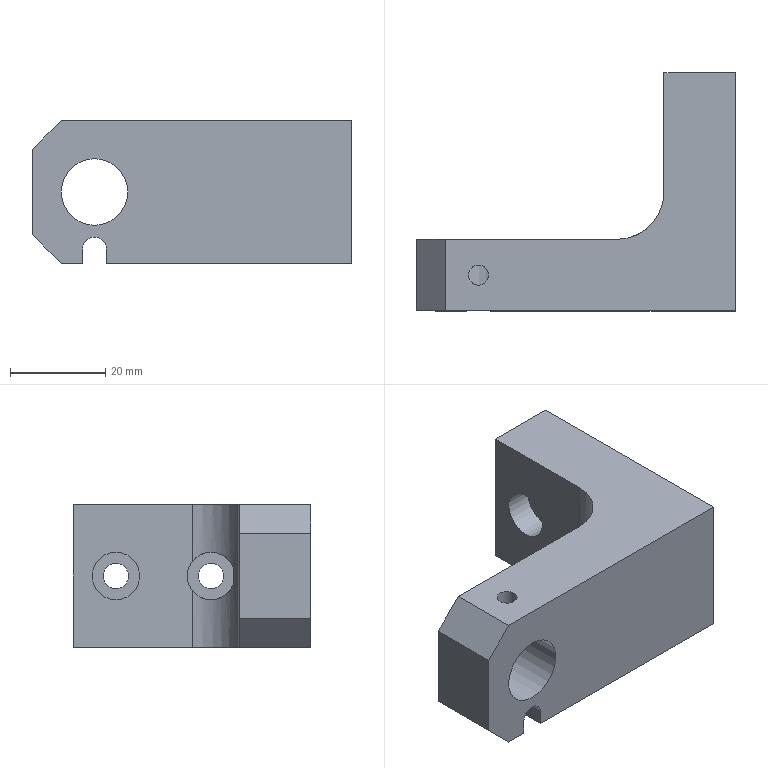Part | NX | 1 solid | 24 faces | box 67 x 50 x 30 mm | volume 41805 mm3 | plane 16 | cylinder 8 | commonest cylinder face diameters 5.3 x2 10 x2 4.2 x1 5 x1 14 x1 20 x1
STEP:
#1=CARTESIAN_POINT('',(52.,25.,30.));
#2=VERTEX_POINT('',#1);
#3=CARTESIAN_POINT('',(52.,25.,18.));
#4=VERTEX_POINT('',#3);
#5=CARTESIAN_POINT('',(52.,25.,30.));
#6=DIRECTION('',(0.,0.,-1.));
#7=VECTOR('',#6,1.);
#8=LINE('',#5,#7);
#9=EDGE_CURVE('',#2,#4,#8,.T.);
#10=ORIENTED_EDGE('',*,*,#9,.T.);
#11=CARTESIAN_POINT('',(47.,16.34,16.812));
#12=VERTEX_POINT('',#11);
#13=CARTESIAN_POINT('',(52.,25.,18.));
#14=CARTESIAN_POINT('',(52.,24.391,18.813));
#15=CARTESIAN_POINT('',(51.939,23.542,19.417));
#16=CARTESIAN_POINT('',(51.481,21.679,20.05));
#17=CARTESIAN_POINT('',(51.086,20.708,20.067));
#18=CARTESIAN_POINT('',(50.07,19.013,19.67));
#19=CARTESIAN_POINT('',(49.463,18.289,19.274));
#20=CARTESIAN_POINT('',(48.204,17.11,18.237));
#21=CARTESIAN_POINT('',(47.538,16.651,17.611));
#22=CARTESIAN_POINT('',(47.,16.34,16.812));
#23=B_SPLINE_CURVE_WITH_KNOTS('',3,(#13,#14,#15,#16,#17,#18,#19,#20,#21,#22),.UNSPECIFIED.,.F.,.F.,(4,2,2,2,4),(0.,0.25,0.5,0.75,1.),.UNSPECIFIED.);
#24=EDGE_CURVE('',#4,#12,#23,.T.);
#25=ORIENTED_EDGE('',*,*,#24,.T.);
#26=CARTESIAN_POINT('',(47.,16.34,13.188));
#27=VERTEX_POINT('',#26);
#28=CARTESIAN_POINT('',(47.,16.34,30.));
#29=DIRECTION('',(0.,0.,1.));
#30=VECTOR('',#29,1.);
#31=LINE('',#28,#30);
#32=EDGE_CURVE('',#27,#12,#31,.T.);
#33=ORIENTED_EDGE('',*,*,#32,.F.);
#34=CARTESIAN_POINT('',(52.,25.,12.));
#35=VERTEX_POINT('',#34);
#36=CARTESIAN_POINT('',(47.,16.34,13.188));
#37=CARTESIAN_POINT('',(47.541,16.652,12.385));
#38=CARTESIAN_POINT('',(48.202,17.109,11.764));
#39=CARTESIAN_POINT('',(49.461,18.287,10.728));
#40=CARTESIAN_POINT('',(50.071,19.015,10.33));
#41=CARTESIAN_POINT('',(51.082,20.701,9.934));
#42=CARTESIAN_POINT('',(51.478,21.67,9.948));
#43=CARTESIAN_POINT('',(51.939,23.538,10.58));
#44=CARTESIAN_POINT('',(52.,24.389,11.185));
#45=CARTESIAN_POINT('',(52.,25.,12.));
#46=B_SPLINE_CURVE_WITH_KNOTS('',3,(#36,#37,#38,#39,#40,#41,#42,#43,#44,#45),.UNSPECIFIED.,.F.,.F.,(4,2,2,2,4),(0.,0.25,0.5,0.75,1.),.UNSPECIFIED.);
#47=EDGE_CURVE('',#27,#35,#46,.T.);
#48=ORIENTED_EDGE('',*,*,#47,.T.);
#49=CARTESIAN_POINT('',(52.,25.,0.));
#50=VERTEX_POINT('',#49);
#51=CARTESIAN_POINT('',(52.,25.,30.));
#52=DIRECTION('',(0.,0.,-1.));
#53=VECTOR('',#52,1.);
#54=LINE('',#51,#53);
#55=EDGE_CURVE('',#35,#50,#54,.T.);
#56=ORIENTED_EDGE('',*,*,#55,.T.);
#57=CARTESIAN_POINT('',(42.,15.,0.));
#58=VERTEX_POINT('',#57);
#59=CARTESIAN_POINT('',(42.,25.,0.));
#60=DIRECTION('',(0.,0.,1.));
#61=DIRECTION('',(-1.,0.,0.));
#62=AXIS2_PLACEMENT_3D('',#59,#60,#61);
#63=CIRCLE('',#62,10.);
#64=EDGE_CURVE('',#58,#50,#63,.T.);
#65=ORIENTED_EDGE('',*,*,#64,.F.);
#66=CARTESIAN_POINT('',(42.,15.,30.));
#67=VERTEX_POINT('',#66);
#68=CARTESIAN_POINT('',(42.,15.,30.));
#69=DIRECTION('',(0.,0.,-1.));
#70=VECTOR('',#69,1.);
#71=LINE('',#68,#70);
#72=EDGE_CURVE('',#67,#58,#71,.T.);
#73=ORIENTED_EDGE('',*,*,#72,.F.);
#74=CARTESIAN_POINT('',(42.,25.,30.));
#75=DIRECTION('',(0.,0.,1.));
#76=DIRECTION('',(-1.,0.,0.));
#77=AXIS2_PLACEMENT_3D('',#74,#75,#76);
#78=CIRCLE('',#77,10.);
#79=EDGE_CURVE('',#67,#2,#78,.T.);
#80=ORIENTED_EDGE('',*,*,#79,.T.);
#81=EDGE_LOOP('',(#10,#25,#33,#48,#56,#65,#73,#80));
#82=FACE_OUTER_BOUND('',#81,.T.);
#83=CARTESIAN_POINT('',(42.,25.,30.));
#84=DIRECTION('',(0.,0.,-1.));
#85=DIRECTION('',(1.,0.,0.));
#86=AXIS2_PLACEMENT_3D('',#83,#84,#85);
#87=CYLINDRICAL_SURFACE('',#86,10.);
#88=ADVANCED_FACE('',(#82),#87,.F.);
#89=CARTESIAN_POINT('',(67.,21.,17.65));
#90=VERTEX_POINT('',#89);
#91=CARTESIAN_POINT('',(67.,21.,15.));
#92=DIRECTION('',(-1.,0.,0.));
#93=DIRECTION('',(0.,0.,1.));
#94=AXIS2_PLACEMENT_3D('',#91,#92,#93);
#95=CIRCLE('',#94,2.65);
#96=EDGE_CURVE('',#90,#90,#95,.T.);
#97=ORIENTED_EDGE('',*,*,#96,.F.);
#98=EDGE_LOOP('',(#97));
#99=FACE_BOUND('',#98,.T.);
#100=CARTESIAN_POINT('',(57.7,21.,17.65));
#101=VERTEX_POINT('',#100);
#102=CARTESIAN_POINT('',(57.7,21.,15.));
#103=DIRECTION('',(1.,0.,0.));
#104=DIRECTION('',(0.,0.,1.));
#105=AXIS2_PLACEMENT_3D('',#102,#103,#104);
#106=CIRCLE('',#105,2.65);
#107=EDGE_CURVE('',#101,#101,#106,.T.);
#108=ORIENTED_EDGE('',*,*,#107,.F.);
#109=EDGE_LOOP('',(#108));
#110=FACE_BOUND('',#109,.T.);
#111=CARTESIAN_POINT('',(47.,21.,15.));
#112=DIRECTION('',(1.,0.,0.));
#113=DIRECTION('',(0.,0.,1.));
#114=AXIS2_PLACEMENT_3D('',#111,#112,#113);
#115=CYLINDRICAL_SURFACE('',#114,2.65);
#116=ADVANCED_FACE('',(#99,#110),#115,.F.);
#117=CARTESIAN_POINT('',(67.,41.,17.65));
#118=VERTEX_POINT('',#117);
#119=CARTESIAN_POINT('',(67.,41.,15.));
#120=DIRECTION('',(1.,0.,0.));
#121=DIRECTION('',(0.,0.,1.));
#122=AXIS2_PLACEMENT_3D('',#119,#120,#121);
#123=CIRCLE('',#122,2.65);
#124=EDGE_CURVE('',#118,#118,#123,.T.);
#125=ORIENTED_EDGE('',*,*,#124,.T.);
#126=EDGE_LOOP('',(#125));
#127=FACE_BOUND('',#126,.T.);
#128=CARTESIAN_POINT('',(57.7,41.,17.65));
#129=VERTEX_POINT('',#128);
#130=CARTESIAN_POINT('',(57.7,41.,15.));
#131=DIRECTION('',(-1.,0.,0.));
#132=DIRECTION('',(0.,0.,1.));
#133=AXIS2_PLACEMENT_3D('',#130,#131,#132);
#134=CIRCLE('',#133,2.65);
#135=EDGE_CURVE('',#129,#129,#134,.T.);
#136=ORIENTED_EDGE('',*,*,#135,.T.);
#137=EDGE_LOOP('',(#136));
#138=FACE_BOUND('',#137,.T.);
#139=CARTESIAN_POINT('',(47.,41.,15.));
#140=DIRECTION('',(1.,0.,0.));
#141=DIRECTION('',(0.,0.,1.));
#142=AXIS2_PLACEMENT_3D('',#139,#140,#141);
#143=CYLINDRICAL_SURFACE('',#142,2.65);
#144=ADVANCED_FACE('',(#127,#138),#143,.F.);
#145=ORIENTED_EDGE('',*,*,#96,.T.);
#146=EDGE_LOOP('',(#145));
#147=FACE_BOUND('',#146,.T.);
#148=CARTESIAN_POINT('',(67.,50.,0.));
#149=VERTEX_POINT('',#148);
#150=CARTESIAN_POINT('',(67.,0.,0.));
#151=VERTEX_POINT('',#150);
#152=CARTESIAN_POINT('',(67.,50.,0.));
#153=DIRECTION('',(0.,-1.,0.));
#154=VECTOR('',#153,1.);
#155=LINE('',#152,#154);
#156=EDGE_CURVE('',#149,#151,#155,.T.);
#157=ORIENTED_EDGE('',*,*,#156,.F.);
#158=CARTESIAN_POINT('',(67.,50.,30.));
#159=VERTEX_POINT('',#158);
#160=CARTESIAN_POINT('',(67.,50.,30.));
#161=DIRECTION('',(0.,0.,-1.));
#162=VECTOR('',#161,1.);
#163=LINE('',#160,#162);
#164=EDGE_CURVE('',#159,#149,#163,.T.);
#165=ORIENTED_EDGE('',*,*,#164,.F.);
#166=CARTESIAN_POINT('',(67.,0.,30.));
#167=VERTEX_POINT('',#166);
#168=CARTESIAN_POINT('',(67.,50.,30.));
#169=DIRECTION('',(0.,-1.,0.));
#170=VECTOR('',#169,1.);
#171=LINE('',#168,#170);
#172=EDGE_CURVE('',#159,#167,#171,.T.);
#173=ORIENTED_EDGE('',*,*,#172,.T.);
#174=CARTESIAN_POINT('',(67.,0.,30.));
#175=DIRECTION('',(0.,0.,-1.));
#176=VECTOR('',#175,1.);
#177=LINE('',#174,#176);
#178=EDGE_CURVE('',#167,#151,#177,.T.);
#179=ORIENTED_EDGE('',*,*,#178,.T.);
#180=EDGE_LOOP('',(#157,#165,#173,#179));
#181=FACE_BOUND('',#180,.T.);
#182=ORIENTED_EDGE('',*,*,#124,.F.);
#183=EDGE_LOOP('',(#182));
#184=FACE_BOUND('',#183,.T.);
#185=CARTESIAN_POINT('',(67.,50.,30.));
#186=DIRECTION('',(1.,0.,0.));
#187=DIRECTION('',(0.,0.,1.));
#188=AXIS2_PLACEMENT_3D('',#185,#186,#187);
#189=PLANE('',#188);
#190=ADVANCED_FACE('',(#147,#181,#184),#189,.T.);
#191=CARTESIAN_POINT('',(15.5,0.,0.));
#192=VERTEX_POINT('',#191);
#193=CARTESIAN_POINT('',(15.5,0.,3.));
#194=VERTEX_POINT('',#193);
#195=CARTESIAN_POINT('',(15.5,0.,0.));
#196=DIRECTION('',(0.,0.,1.));
#197=VECTOR('',#196,1.);
#198=LINE('',#195,#197);
#199=EDGE_CURVE('',#192,#194,#198,.T.);
#200=ORIENTED_EDGE('',*,*,#199,.F.);
#201=CARTESIAN_POINT('',(6.,0.,0.));
#202=DIRECTION('',(-1.,0.,0.));
#203=VECTOR('',#202,1.);
#204=LINE('',#201,#203);
#205=EDGE_CURVE('',#151,#192,#204,.T.);
#206=ORIENTED_EDGE('',*,*,#205,.F.);
#207=ORIENTED_EDGE('',*,*,#178,.F.);
#208=CARTESIAN_POINT('',(6.,0.,30.));
#209=VERTEX_POINT('',#208);
#210=CARTESIAN_POINT('',(67.,0.,30.));
#211=DIRECTION('',(-1.,0.,0.));
#212=VECTOR('',#211,1.);
#213=LINE('',#210,#212);
#214=EDGE_CURVE('',#167,#209,#213,.T.);
#215=ORIENTED_EDGE('',*,*,#214,.T.);
#216=CARTESIAN_POINT('',(0.,0.,24.));
#217=VERTEX_POINT('',#216);
#218=CARTESIAN_POINT('',(6.,0.,30.));
#219=DIRECTION('',(-0.7071,0.,-0.7071));
#220=VECTOR('',#219,1.);
#221=LINE('',#218,#220);
#222=EDGE_CURVE('',#209,#217,#221,.T.);
#223=ORIENTED_EDGE('',*,*,#222,.T.);
#224=CARTESIAN_POINT('',(0.,0.,6.));
#225=VERTEX_POINT('',#224);
#226=CARTESIAN_POINT('',(0.,0.,30.));
#227=DIRECTION('',(0.,0.,-1.));
#228=VECTOR('',#227,1.);
#229=LINE('',#226,#228);
#230=EDGE_CURVE('',#217,#225,#229,.T.);
#231=ORIENTED_EDGE('',*,*,#230,.T.);
#232=CARTESIAN_POINT('',(6.,0.,0.));
#233=VERTEX_POINT('',#232);
#234=CARTESIAN_POINT('',(-9.,0.,15.));
#235=DIRECTION('',(0.7071,0.,-0.7071));
#236=VECTOR('',#235,1.);
#237=LINE('',#234,#236);
#238=EDGE_CURVE('',#225,#233,#237,.T.);
#239=ORIENTED_EDGE('',*,*,#238,.T.);
#240=CARTESIAN_POINT('',(10.5,0.,0.));
#241=VERTEX_POINT('',#240);
#242=CARTESIAN_POINT('',(6.,0.,0.));
#243=DIRECTION('',(-1.,0.,0.));
#244=VECTOR('',#243,1.);
#245=LINE('',#242,#244);
#246=EDGE_CURVE('',#241,#233,#245,.T.);
#247=ORIENTED_EDGE('',*,*,#246,.F.);
#248=CARTESIAN_POINT('',(10.5,0.,3.));
#249=VERTEX_POINT('',#248);
#250=CARTESIAN_POINT('',(10.5,0.,3.));
#251=DIRECTION('',(0.,0.,-1.));
#252=VECTOR('',#251,1.);
#253=LINE('',#250,#252);
#254=EDGE_CURVE('',#249,#241,#253,.T.);
#255=ORIENTED_EDGE('',*,*,#254,.F.);
#256=CARTESIAN_POINT('',(13.,0.,3.));
#257=DIRECTION('',(0.,-1.,0.));
#258=DIRECTION('',(0.,0.,1.));
#259=AXIS2_PLACEMENT_3D('',#256,#257,#258);
#260=CIRCLE('',#259,2.5);
#261=EDGE_CURVE('',#194,#249,#260,.T.);
#262=ORIENTED_EDGE('',*,*,#261,.F.);
#263=EDGE_LOOP('',(#200,#206,#207,#215,#223,#231,#239,#247,#255,#262));
#264=FACE_BOUND('',#263,.T.);
#265=CARTESIAN_POINT('',(13.,0.,22.));
#266=VERTEX_POINT('',#265);
#267=CARTESIAN_POINT('',(13.,0.,15.));
#268=DIRECTION('',(0.,1.,0.));
#269=DIRECTION('',(0.,0.,1.));
#270=AXIS2_PLACEMENT_3D('',#267,#268,#269);
#271=CIRCLE('',#270,7.);
#272=EDGE_CURVE('',#266,#266,#271,.T.);
#273=ORIENTED_EDGE('',*,*,#272,.T.);
#274=EDGE_LOOP('',(#273));
#275=FACE_BOUND('',#274,.T.);
#276=CARTESIAN_POINT('',(6.,0.,30.));
#277=DIRECTION('',(0.,-1.,0.));
#278=DIRECTION('',(0.,0.,1.));
#279=AXIS2_PLACEMENT_3D('',#276,#277,#278);
#280=PLANE('',#279);
#281=ADVANCED_FACE('',(#264,#275),#280,.T.);
#282=CARTESIAN_POINT('',(10.5,15.,0.));
#283=VERTEX_POINT('',#282);
#284=CARTESIAN_POINT('',(10.5,15.,3.));
#285=VERTEX_POINT('',#284);
#286=CARTESIAN_POINT('',(10.5,15.,30.));
#287=DIRECTION('',(0.,0.,1.));
#288=VECTOR('',#287,1.);
#289=LINE('',#286,#288);
#290=EDGE_CURVE('',#283,#285,#289,.T.);
#291=ORIENTED_EDGE('',*,*,#290,.F.);
#292=CARTESIAN_POINT('',(6.,15.,0.));
#293=VERTEX_POINT('',#292);
#294=CARTESIAN_POINT('',(0.,15.,0.));
#295=DIRECTION('',(1.,0.,0.));
#296=VECTOR('',#295,1.);
#297=LINE('',#294,#296);
#298=EDGE_CURVE('',#293,#283,#297,.T.);
#299=ORIENTED_EDGE('',*,*,#298,.F.);
#300=CARTESIAN_POINT('',(0.,15.,6.));
#301=VERTEX_POINT('',#300);
#302=CARTESIAN_POINT('',(-12.,15.,18.));
#303=DIRECTION('',(-0.7071,0.,0.7071));
#304=VECTOR('',#303,1.);
#305=LINE('',#302,#304);
#306=EDGE_CURVE('',#293,#301,#305,.T.);
#307=ORIENTED_EDGE('',*,*,#306,.T.);
#308=CARTESIAN_POINT('',(0.,15.,24.));
#309=VERTEX_POINT('',#308);
#310=CARTESIAN_POINT('',(0.,15.,30.));
#311=DIRECTION('',(0.,0.,-1.));
#312=VECTOR('',#311,1.);
#313=LINE('',#310,#312);
#314=EDGE_CURVE('',#309,#301,#313,.T.);
#315=ORIENTED_EDGE('',*,*,#314,.F.);
#316=CARTESIAN_POINT('',(6.,15.,30.));
#317=VERTEX_POINT('',#316);
#318=CARTESIAN_POINT('',(3.,15.,27.));
#319=DIRECTION('',(0.7071,0.,0.7071));
#320=VECTOR('',#319,1.);
#321=LINE('',#318,#320);
#322=EDGE_CURVE('',#309,#317,#321,.T.);
#323=ORIENTED_EDGE('',*,*,#322,.T.);
#324=CARTESIAN_POINT('',(6.,15.,30.));
#325=DIRECTION('',(1.,0.,0.));
#326=VECTOR('',#325,1.);
#327=LINE('',#324,#326);
#328=EDGE_CURVE('',#317,#67,#327,.T.);
#329=ORIENTED_EDGE('',*,*,#328,.T.);
#330=ORIENTED_EDGE('',*,*,#72,.T.);
#331=CARTESIAN_POINT('',(15.5,15.,0.));
#332=VERTEX_POINT('',#331);
#333=CARTESIAN_POINT('',(0.,15.,0.));
#334=DIRECTION('',(1.,0.,0.));
#335=VECTOR('',#334,1.);
#336=LINE('',#333,#335);
#337=EDGE_CURVE('',#332,#58,#336,.T.);
#338=ORIENTED_EDGE('',*,*,#337,.F.);
#339=CARTESIAN_POINT('',(15.5,15.,3.));
#340=VERTEX_POINT('',#339);
#341=CARTESIAN_POINT('',(15.5,15.,30.));
#342=DIRECTION('',(0.,0.,-1.));
#343=VECTOR('',#342,1.);
#344=LINE('',#341,#343);
#345=EDGE_CURVE('',#340,#332,#344,.T.);
#346=ORIENTED_EDGE('',*,*,#345,.F.);
#347=CARTESIAN_POINT('',(13.,15.,3.));
#348=DIRECTION('',(0.,1.,0.));
#349=DIRECTION('',(0.,0.,1.));
#350=AXIS2_PLACEMENT_3D('',#347,#348,#349);
#351=CIRCLE('',#350,2.5);
#352=EDGE_CURVE('',#285,#340,#351,.T.);
#353=ORIENTED_EDGE('',*,*,#352,.F.);
#354=EDGE_LOOP('',(#291,#299,#307,#315,#323,#329,#330,#338,#346,#353));
#355=FACE_BOUND('',#354,.T.);
#356=CARTESIAN_POINT('',(13.,15.,22.));
#357=VERTEX_POINT('',#356);
#358=CARTESIAN_POINT('',(13.,15.,15.));
#359=DIRECTION('',(0.,-1.,0.));
#360=DIRECTION('',(0.,0.,1.));
#361=AXIS2_PLACEMENT_3D('',#358,#359,#360);
#362=CIRCLE('',#361,7.);
#363=EDGE_CURVE('',#357,#357,#362,.T.);
#364=ORIENTED_EDGE('',*,*,#363,.T.);
#365=EDGE_LOOP('',(#364));
#366=FACE_BOUND('',#365,.T.);
#367=CARTESIAN_POINT('',(0.,15.,30.));
#368=DIRECTION('',(0.,1.,0.));
#369=DIRECTION('',(0.,0.,-1.));
#370=AXIS2_PLACEMENT_3D('',#367,#368,#369);
#371=PLANE('',#370);
#372=ADVANCED_FACE('',(#355,#366),#371,.T.);
#373=CARTESIAN_POINT('',(15.5,20.,0.));
#374=DIRECTION('',(0.,-1.,0.));
#375=VECTOR('',#374,1.);
#376=LINE('',#373,#375);
#377=EDGE_CURVE('',#332,#192,#376,.T.);
#378=ORIENTED_EDGE('',*,*,#377,.F.);
#379=ORIENTED_EDGE('',*,*,#337,.T.);
#380=ORIENTED_EDGE('',*,*,#64,.T.);
#381=CARTESIAN_POINT('',(52.,50.,0.));
#382=VERTEX_POINT('',#381);
#383=CARTESIAN_POINT('',(52.,25.,0.));
#384=DIRECTION('',(0.,1.,0.));
#385=VECTOR('',#384,1.);
#386=LINE('',#383,#385);
#387=EDGE_CURVE('',#50,#382,#386,.T.);
#388=ORIENTED_EDGE('',*,*,#387,.T.);
#389=CARTESIAN_POINT('',(52.,50.,0.));
#390=DIRECTION('',(1.,0.,0.));
#391=VECTOR('',#390,1.);
#392=LINE('',#389,#391);
#393=EDGE_CURVE('',#382,#149,#392,.T.);
#394=ORIENTED_EDGE('',*,*,#393,.T.);
#395=ORIENTED_EDGE('',*,*,#156,.T.);
#396=ORIENTED_EDGE('',*,*,#205,.T.);
#397=EDGE_LOOP('',(#378,#379,#380,#388,#394,#395,#396));
#398=FACE_OUTER_BOUND('',#397,.T.);
#399=CARTESIAN_POINT('',(42.,25.,0.));
#400=DIRECTION('',(0.,0.,1.));
#401=DIRECTION('',(-1.,0.,0.));
#402=AXIS2_PLACEMENT_3D('',#399,#400,#401);
#403=PLANE('',#402);
#404=ADVANCED_FACE('',(#398),#403,.F.);
#405=CARTESIAN_POINT('',(15.1,7.5,30.));
#406=VERTEX_POINT('',#405);
#407=CARTESIAN_POINT('',(13.,7.5,30.));
#408=DIRECTION('',(0.,0.,-1.));
#409=DIRECTION('',(1.,0.,0.));
#410=AXIS2_PLACEMENT_3D('',#407,#408,#409);
#411=CIRCLE('',#410,2.1);
#412=EDGE_CURVE('',#406,#406,#411,.T.);
#413=ORIENTED_EDGE('',*,*,#412,.F.);
#414=EDGE_LOOP('',(#413));
#415=FACE_BOUND('',#414,.T.);
#416=CARTESIAN_POINT('',(10.9,7.5,21.678));
#417=VERTEX_POINT('',#416);
#418=CARTESIAN_POINT('',(10.9,7.5,21.678));
#419=CARTESIAN_POINT('',(10.9,7.729,21.678));
#420=CARTESIAN_POINT('',(10.939,7.961,21.69));
#421=CARTESIAN_POINT('',(11.012,8.177,21.712));
#422=CARTESIAN_POINT('',(11.086,8.393,21.734));
#423=CARTESIAN_POINT('',(11.196,8.598,21.765));
#424=CARTESIAN_POINT('',(11.333,8.778,21.799));
#425=CARTESIAN_POINT('',(11.475,8.962,21.833));
#426=CARTESIAN_POINT('',(11.65,9.125,21.871));
#427=CARTESIAN_POINT('',(11.844,9.253,21.904));
#428=CARTESIAN_POINT('',(12.043,9.384,21.937));
#429=CARTESIAN_POINT('',(12.268,9.483,21.966));
#430=CARTESIAN_POINT('',(12.501,9.54,21.982));
#431=CARTESIAN_POINT('',(12.727,9.595,21.998));
#432=CARTESIAN_POINT('',(12.967,9.613,22.004));
#433=CARTESIAN_POINT('',(13.199,9.591,21.997));
#434=CARTESIAN_POINT('',(13.423,9.569,21.991));
#435=CARTESIAN_POINT('',(13.647,9.51,21.973));
#436=CARTESIAN_POINT('',(13.852,9.419,21.948));
#437=CARTESIAN_POINT('',(14.06,9.327,21.922));
#438=CARTESIAN_POINT('',(14.254,9.2,21.889));
#439=CARTESIAN_POINT('',(14.421,9.047,21.854));
#440=CARTESIAN_POINT('',(14.593,8.888,21.819));
#441=CARTESIAN_POINT('',(14.741,8.697,21.781));
#442=CARTESIAN_POINT('',(14.852,8.49,21.751));
#443=CARTESIAN_POINT('',(14.964,8.28,21.72));
#444=CARTESIAN_POINT('',(15.042,8.047,21.696));
#445=CARTESIAN_POINT('',(15.077,7.81,21.685));
#446=CARTESIAN_POINT('',(15.111,7.583,21.674));
#447=CARTESIAN_POINT('',(15.107,7.345,21.676));
#448=CARTESIAN_POINT('',(15.065,7.119,21.688));
#449=CARTESIAN_POINT('',(15.024,6.898,21.701));
#450=CARTESIAN_POINT('',(14.947,6.682,21.725));
#451=CARTESIAN_POINT('',(14.839,6.487,21.754));
#452=CARTESIAN_POINT('',(14.729,6.286,21.784));
#453=CARTESIAN_POINT('',(14.584,6.103,21.821));
#454=CARTESIAN_POINT('',(14.416,5.949,21.855));
#455=CARTESIAN_POINT('',(14.241,5.789,21.891));
#456=CARTESIAN_POINT('',(14.036,5.658,21.926));
#457=CARTESIAN_POINT('',(13.816,5.565,21.952));
#458=CARTESIAN_POINT('',(13.599,5.473,21.978));
#459=CARTESIAN_POINT('',(13.361,5.418,21.995));
#460=CARTESIAN_POINT('',(13.124,5.404,21.999));
#461=CARTESIAN_POINT('',(12.896,5.39,22.003));
#462=CARTESIAN_POINT('',(12.662,5.415,21.995));
#463=CARTESIAN_POINT('',(12.443,5.475,21.978));
#464=CARTESIAN_POINT('',(12.226,5.535,21.96));
#465=CARTESIAN_POINT('',(12.016,5.631,21.933));
#466=CARTESIAN_POINT('',(11.83,5.756,21.902));
#467=CARTESIAN_POINT('',(11.638,5.885,21.869));
#468=CARTESIAN_POINT('',(11.466,6.047,21.831));
#469=CARTESIAN_POINT('',(11.327,6.231,21.797));
#470=CARTESIAN_POINT('',(11.183,6.42,21.762));
#471=CARTESIAN_POINT('',(11.07,6.637,21.729));
#472=CARTESIAN_POINT('',(10.998,6.865,21.708));
#473=CARTESIAN_POINT('',(10.934,7.069,21.688));
#474=CARTESIAN_POINT('',(10.9,7.286,21.678));
#475=CARTESIAN_POINT('',(10.9,7.5,21.678));
#476=B_SPLINE_CURVE_WITH_KNOTS('',3,(#418,#419,#420,#421,#422,#423,#424,#425,#426,#427,#428,#429,#430,#431,#432,#433,#434,#435,#436,#437,#438,#439,#440,#441,#442,#443,#444,#445,#446,#447,#448,#449,#450,#451,#452,#453,#454,#455,#456,#457,#458,#459,#460,#461,#462,#463,#464,#465,#466,#467,#468,#469,#470,#471,#472,#473,#474,#475),.UNSPECIFIED.,.T.,.F.,(1,3,3,3,3,3,3,3,3,3,3,3,3,3,3,3,3,3,3,3,3,1),(-0.04857,0.,0.05204,0.104,0.1574,0.212,0.2651,0.3163,0.3682,0.4221,0.4766,0.529,0.58,0.6324,0.6868,0.7408,0.7926,0.8439,0.8969,0.9514,1.,1.052),.UNSPECIFIED.);
#477=EDGE_CURVE('',#417,#417,#476,.T.);
#478=ORIENTED_EDGE('',*,*,#477,.T.);
#479=EDGE_LOOP('',(#478));
#480=FACE_BOUND('',#479,.T.);
#481=CARTESIAN_POINT('',(13.,7.5,35.));
#482=DIRECTION('',(0.,0.,-1.));
#483=DIRECTION('',(1.,0.,0.));
#484=AXIS2_PLACEMENT_3D('',#481,#482,#483);
#485=CYLINDRICAL_SURFACE('',#484,2.1);
#486=ADVANCED_FACE('',(#415,#480),#485,.F.);
#487=CARTESIAN_POINT('',(52.,41.,20.));
#488=VERTEX_POINT('',#487);
#489=CARTESIAN_POINT('',(52.,41.,15.));
#490=DIRECTION('',(1.,0.,0.));
#491=DIRECTION('',(0.,0.,1.));
#492=AXIS2_PLACEMENT_3D('',#489,#490,#491);
#493=CIRCLE('',#492,5.);
#494=EDGE_CURVE('',#488,#488,#493,.T.);
#495=ORIENTED_EDGE('',*,*,#494,.T.);
#496=EDGE_LOOP('',(#495));
#497=FACE_BOUND('',#496,.T.);
#498=ORIENTED_EDGE('',*,*,#55,.F.);
#499=CARTESIAN_POINT('',(52.,21.,15.));
#500=DIRECTION('',(1.,0.,0.));
#501=DIRECTION('',(0.,0.,1.));
#502=AXIS2_PLACEMENT_3D('',#499,#500,#501);
#503=CIRCLE('',#502,5.);
#504=EDGE_CURVE('',#35,#4,#503,.T.);
#505=ORIENTED_EDGE('',*,*,#504,.T.);
#506=ORIENTED_EDGE('',*,*,#9,.F.);
#507=CARTESIAN_POINT('',(52.,50.,30.));
#508=VERTEX_POINT('',#507);
#509=CARTESIAN_POINT('',(52.,25.,30.));
#510=DIRECTION('',(0.,1.,0.));
#511=VECTOR('',#510,1.);
#512=LINE('',#509,#511);
#513=EDGE_CURVE('',#2,#508,#512,.T.);
#514=ORIENTED_EDGE('',*,*,#513,.T.);
#515=CARTESIAN_POINT('',(52.,50.,30.));
#516=DIRECTION('',(0.,0.,-1.));
#517=VECTOR('',#516,1.);
#518=LINE('',#515,#517);
#519=EDGE_CURVE('',#508,#382,#518,.T.);
#520=ORIENTED_EDGE('',*,*,#519,.T.);
#521=ORIENTED_EDGE('',*,*,#387,.F.);
#522=EDGE_LOOP('',(#498,#505,#506,#514,#520,#521));
#523=FACE_BOUND('',#522,.T.);
#524=CARTESIAN_POINT('',(52.,25.,30.));
#525=DIRECTION('',(-1.,0.,0.));
#526=DIRECTION('',(0.,0.,-1.));
#527=AXIS2_PLACEMENT_3D('',#524,#525,#526);
#528=PLANE('',#527);
#529=ADVANCED_FACE('',(#497,#523),#528,.T.);
#530=ORIENTED_EDGE('',*,*,#393,.F.);
#531=ORIENTED_EDGE('',*,*,#519,.F.);
#532=CARTESIAN_POINT('',(52.,50.,30.));
#533=DIRECTION('',(1.,0.,0.));
#534=VECTOR('',#533,1.);
#535=LINE('',#532,#534);
#536=EDGE_CURVE('',#508,#159,#535,.T.);
#537=ORIENTED_EDGE('',*,*,#536,.T.);
#538=ORIENTED_EDGE('',*,*,#164,.T.);
#539=EDGE_LOOP('',(#530,#531,#537,#538));
#540=FACE_OUTER_BOUND('',#539,.T.);
#541=CARTESIAN_POINT('',(52.,50.,30.));
#542=DIRECTION('',(0.,1.,0.));
#543=DIRECTION('',(0.,0.,-1.));
#544=AXIS2_PLACEMENT_3D('',#541,#542,#543);
#545=PLANE('',#544);
#546=ADVANCED_FACE('',(#540),#545,.T.);
#547=ORIENTED_EDGE('',*,*,#314,.T.);
#548=CARTESIAN_POINT('',(0.,0.,6.));
#549=DIRECTION('',(0.,-1.,0.));
#550=VECTOR('',#549,1.);
#551=LINE('',#548,#550);
#552=EDGE_CURVE('',#301,#225,#551,.T.);
#553=ORIENTED_EDGE('',*,*,#552,.T.);
#554=ORIENTED_EDGE('',*,*,#230,.F.);
#555=CARTESIAN_POINT('',(0.,0.,24.));
#556=DIRECTION('',(0.,1.,0.));
#557=VECTOR('',#556,1.);
#558=LINE('',#555,#557);
#559=EDGE_CURVE('',#217,#309,#558,.T.);
#560=ORIENTED_EDGE('',*,*,#559,.T.);
#561=EDGE_LOOP('',(#547,#553,#554,#560));
#562=FACE_OUTER_BOUND('',#561,.T.);
#563=CARTESIAN_POINT('',(0.,0.,30.));
#564=DIRECTION('',(-1.,0.,0.));
#565=DIRECTION('',(0.,0.,-1.));
#566=AXIS2_PLACEMENT_3D('',#563,#564,#565);
#567=PLANE('',#566);
#568=ADVANCED_FACE('',(#562),#567,.T.);
#569=ORIENTED_EDGE('',*,*,#412,.T.);
#570=EDGE_LOOP('',(#569));
#571=FACE_BOUND('',#570,.T.);
#572=ORIENTED_EDGE('',*,*,#328,.F.);
#573=CARTESIAN_POINT('',(6.,25.,30.));
#574=DIRECTION('',(0.,-1.,0.));
#575=VECTOR('',#574,1.);
#576=LINE('',#573,#575);
#577=EDGE_CURVE('',#317,#209,#576,.T.);
#578=ORIENTED_EDGE('',*,*,#577,.T.);
#579=ORIENTED_EDGE('',*,*,#214,.F.);
#580=ORIENTED_EDGE('',*,*,#172,.F.);
#581=ORIENTED_EDGE('',*,*,#536,.F.);
#582=ORIENTED_EDGE('',*,*,#513,.F.);
#583=ORIENTED_EDGE('',*,*,#79,.F.);
#584=EDGE_LOOP('',(#572,#578,#579,#580,#581,#582,#583));
#585=FACE_BOUND('',#584,.T.);
#586=CARTESIAN_POINT('',(42.,25.,30.));
#587=DIRECTION('',(0.,0.,1.));
#588=DIRECTION('',(-1.,0.,0.));
#589=AXIS2_PLACEMENT_3D('',#586,#587,#588);
#590=PLANE('',#589);
#591=ADVANCED_FACE('',(#571,#585),#590,.T.);
#592=ORIENTED_EDGE('',*,*,#298,.T.);
#593=CARTESIAN_POINT('',(10.5,20.,0.));
#594=DIRECTION('',(0.,-1.,0.));
#595=VECTOR('',#594,1.);
#596=LINE('',#593,#595);
#597=EDGE_CURVE('',#283,#241,#596,.T.);
#598=ORIENTED_EDGE('',*,*,#597,.T.);
#599=ORIENTED_EDGE('',*,*,#246,.T.);
#600=CARTESIAN_POINT('',(6.,15.,0.));
#601=DIRECTION('',(0.,1.,0.));
#602=VECTOR('',#601,1.);
#603=LINE('',#600,#602);
#604=EDGE_CURVE('',#233,#293,#603,.T.);
#605=ORIENTED_EDGE('',*,*,#604,.T.);
#606=EDGE_LOOP('',(#592,#598,#599,#605));
#607=FACE_OUTER_BOUND('',#606,.T.);
#608=CARTESIAN_POINT('',(42.,25.,0.));
#609=DIRECTION('',(0.,0.,1.));
#610=DIRECTION('',(-1.,0.,0.));
#611=AXIS2_PLACEMENT_3D('',#608,#609,#610);
#612=PLANE('',#611);
#613=ADVANCED_FACE('',(#607),#612,.F.);
#614=ORIENTED_EDGE('',*,*,#238,.F.);
#615=ORIENTED_EDGE('',*,*,#552,.F.);
#616=ORIENTED_EDGE('',*,*,#306,.F.);
#617=ORIENTED_EDGE('',*,*,#604,.F.);
#618=EDGE_LOOP('',(#614,#615,#616,#617));
#619=FACE_OUTER_BOUND('',#618,.T.);
#620=CARTESIAN_POINT('',(6.,25.,0.));
#621=DIRECTION('',(-0.7071,0.,-0.7071));
#622=DIRECTION('',(0.,1.,0.));
#623=AXIS2_PLACEMENT_3D('',#620,#621,#622);
#624=PLANE('',#623);
#625=ADVANCED_FACE('',(#619),#624,.T.);
#626=ORIENTED_EDGE('',*,*,#222,.F.);
#627=ORIENTED_EDGE('',*,*,#577,.F.);
#628=ORIENTED_EDGE('',*,*,#322,.F.);
#629=ORIENTED_EDGE('',*,*,#559,.F.);
#630=EDGE_LOOP('',(#626,#627,#628,#629));
#631=FACE_OUTER_BOUND('',#630,.T.);
#632=CARTESIAN_POINT('',(0.,0.,24.));
#633=DIRECTION('',(0.7071,0.,-0.7071));
#634=DIRECTION('',(0.,-1.,0.));
#635=AXIS2_PLACEMENT_3D('',#632,#633,#634);
#636=PLANE('',#635);
#637=ADVANCED_FACE('',(#631),#636,.F.);
#638=ORIENTED_EDGE('',*,*,#363,.F.);
#639=EDGE_LOOP('',(#638));
#640=FACE_BOUND('',#639,.T.);
#641=ORIENTED_EDGE('',*,*,#477,.F.);
#642=EDGE_LOOP('',(#641));
#643=FACE_BOUND('',#642,.T.);
#644=ORIENTED_EDGE('',*,*,#272,.F.);
#645=EDGE_LOOP('',(#644));
#646=FACE_BOUND('',#645,.T.);
#647=CARTESIAN_POINT('',(13.,20.,15.));
#648=DIRECTION('',(0.,-1.,0.));
#649=DIRECTION('',(0.,0.,1.));
#650=AXIS2_PLACEMENT_3D('',#647,#648,#649);
#651=CYLINDRICAL_SURFACE('',#650,7.);
#652=ADVANCED_FACE('',(#640,#643,#646),#651,.F.);
#653=ORIENTED_EDGE('',*,*,#352,.T.);
#654=CARTESIAN_POINT('',(15.5,20.,3.));
#655=DIRECTION('',(0.,1.,0.));
#656=VECTOR('',#655,1.);
#657=LINE('',#654,#656);
#658=EDGE_CURVE('',#194,#340,#657,.T.);
#659=ORIENTED_EDGE('',*,*,#658,.F.);
#660=ORIENTED_EDGE('',*,*,#261,.T.);
#661=CARTESIAN_POINT('',(10.5,20.,3.));
#662=DIRECTION('',(0.,1.,0.));
#663=VECTOR('',#662,1.);
#664=LINE('',#661,#663);
#665=EDGE_CURVE('',#249,#285,#664,.T.);
#666=ORIENTED_EDGE('',*,*,#665,.T.);
#667=EDGE_LOOP('',(#653,#659,#660,#666));
#668=FACE_OUTER_BOUND('',#667,.T.);
#669=CARTESIAN_POINT('',(13.,20.,3.));
#670=DIRECTION('',(0.,-1.,0.));
#671=DIRECTION('',(0.,0.,1.));
#672=AXIS2_PLACEMENT_3D('',#669,#670,#671);
#673=CYLINDRICAL_SURFACE('',#672,2.5);
#674=ADVANCED_FACE('',(#668),#673,.F.);
#675=ORIENTED_EDGE('',*,*,#290,.T.);
#676=ORIENTED_EDGE('',*,*,#665,.F.);
#677=ORIENTED_EDGE('',*,*,#254,.T.);
#678=ORIENTED_EDGE('',*,*,#597,.F.);
#679=EDGE_LOOP('',(#675,#676,#677,#678));
#680=FACE_OUTER_BOUND('',#679,.T.);
#681=CARTESIAN_POINT('',(10.5,20.,3.));
#682=DIRECTION('',(-1.,0.,0.));
#683=DIRECTION('',(0.,0.,-1.));
#684=AXIS2_PLACEMENT_3D('',#681,#682,#683);
#685=PLANE('',#684);
#686=ADVANCED_FACE('',(#680),#685,.F.);
#687=ORIENTED_EDGE('',*,*,#345,.T.);
#688=ORIENTED_EDGE('',*,*,#377,.T.);
#689=ORIENTED_EDGE('',*,*,#199,.T.);
#690=ORIENTED_EDGE('',*,*,#658,.T.);
#691=EDGE_LOOP('',(#687,#688,#689,#690));
#692=FACE_OUTER_BOUND('',#691,.T.);
#693=CARTESIAN_POINT('',(15.5,20.,0.));
#694=DIRECTION('',(1.,0.,0.));
#695=DIRECTION('',(0.,0.,1.));
#696=AXIS2_PLACEMENT_3D('',#693,#694,#695);
#697=PLANE('',#696);
#698=ADVANCED_FACE('',(#692),#697,.F.);
#699=CARTESIAN_POINT('',(57.7,41.,20.));
#700=VERTEX_POINT('',#699);
#701=CARTESIAN_POINT('',(57.7,41.,15.));
#702=DIRECTION('',(-1.,0.,0.));
#703=DIRECTION('',(0.,0.,1.));
#704=AXIS2_PLACEMENT_3D('',#701,#702,#703);
#705=CIRCLE('',#704,5.);
#706=EDGE_CURVE('',#700,#700,#705,.T.);
#707=ORIENTED_EDGE('',*,*,#706,.T.);
#708=EDGE_LOOP('',(#707));
#709=FACE_BOUND('',#708,.T.);
#710=ORIENTED_EDGE('',*,*,#135,.F.);
#711=EDGE_LOOP('',(#710));
#712=FACE_BOUND('',#711,.T.);
#713=CARTESIAN_POINT('',(57.7,41.,15.));
#714=DIRECTION('',(-1.,0.,0.));
#715=DIRECTION('',(0.,0.,-1.));
#716=AXIS2_PLACEMENT_3D('',#713,#714,#715);
#717=PLANE('',#716);
#718=ADVANCED_FACE('',(#709,#712),#717,.T.);
#719=ORIENTED_EDGE('',*,*,#494,.F.);
#720=EDGE_LOOP('',(#719));
#721=FACE_BOUND('',#720,.T.);
#722=ORIENTED_EDGE('',*,*,#706,.F.);
#723=EDGE_LOOP('',(#722));
#724=FACE_BOUND('',#723,.T.);
#725=CARTESIAN_POINT('',(47.,41.,15.));
#726=DIRECTION('',(1.,0.,0.));
#727=DIRECTION('',(0.,0.,1.));
#728=AXIS2_PLACEMENT_3D('',#725,#726,#727);
#729=CYLINDRICAL_SURFACE('',#728,5.);
#730=ADVANCED_FACE('',(#721,#724),#729,.F.);
#731=CARTESIAN_POINT('',(57.7,21.,20.));
#732=VERTEX_POINT('',#731);
#733=CARTESIAN_POINT('',(57.7,21.,15.));
#734=DIRECTION('',(-1.,0.,0.));
#735=DIRECTION('',(0.,0.,1.));
#736=AXIS2_PLACEMENT_3D('',#733,#734,#735);
#737=CIRCLE('',#736,5.);
#738=EDGE_CURVE('',#732,#732,#737,.T.);
#739=ORIENTED_EDGE('',*,*,#738,.F.);
#740=EDGE_LOOP('',(#739));
#741=FACE_BOUND('',#740,.T.);
#742=ORIENTED_EDGE('',*,*,#504,.F.);
#743=ORIENTED_EDGE('',*,*,#47,.F.);
#744=CARTESIAN_POINT('',(47.,21.,15.));
#745=DIRECTION('',(1.,0.,0.));
#746=DIRECTION('',(0.,0.,1.));
#747=AXIS2_PLACEMENT_3D('',#744,#745,#746);
#748=CIRCLE('',#747,5.);
#749=EDGE_CURVE('',#12,#27,#748,.T.);
#750=ORIENTED_EDGE('',*,*,#749,.F.);
#751=ORIENTED_EDGE('',*,*,#24,.F.);
#752=EDGE_LOOP('',(#742,#743,#750,#751));
#753=FACE_BOUND('',#752,.T.);
#754=CARTESIAN_POINT('',(47.,21.,15.));
#755=DIRECTION('',(1.,0.,0.));
#756=DIRECTION('',(0.,0.,1.));
#757=AXIS2_PLACEMENT_3D('',#754,#755,#756);
#758=CYLINDRICAL_SURFACE('',#757,5.);
#759=ADVANCED_FACE('',(#741,#753),#758,.F.);
#760=ORIENTED_EDGE('',*,*,#32,.T.);
#761=ORIENTED_EDGE('',*,*,#749,.T.);
#762=EDGE_LOOP('',(#760,#761));
#763=FACE_OUTER_BOUND('',#762,.T.);
#764=CARTESIAN_POINT('',(47.,21.,15.));
#765=DIRECTION('',(-1.,0.,0.));
#766=DIRECTION('',(0.,0.,-1.));
#767=AXIS2_PLACEMENT_3D('',#764,#765,#766);
#768=PLANE('',#767);
#769=ADVANCED_FACE('',(#763),#768,.F.);
#770=ORIENTED_EDGE('',*,*,#107,.T.);
#771=EDGE_LOOP('',(#770));
#772=FACE_BOUND('',#771,.T.);
#773=ORIENTED_EDGE('',*,*,#738,.T.);
#774=EDGE_LOOP('',(#773));
#775=FACE_BOUND('',#774,.T.);
#776=CARTESIAN_POINT('',(57.7,21.,15.));
#777=DIRECTION('',(-1.,0.,0.));
#778=DIRECTION('',(0.,0.,-1.));
#779=AXIS2_PLACEMENT_3D('',#776,#777,#778);
#780=PLANE('',#779);
#781=ADVANCED_FACE('',(#772,#775),#780,.T.);
#782=CLOSED_SHELL('',(#88,#116,#144,#190,#281,#372,#404,#486,#529,#546,#568,#591,#613,#625,#637,#652,#674,#686,#698,#718,#730,#759,#769,#781));
#783=MANIFOLD_SOLID_BREP('',#782);
#784=(LENGTH_UNIT()NAMED_UNIT(*)SI_UNIT(.MILLI.,.METRE.));
#785=UNCERTAINTY_MEASURE_WITH_UNIT(LENGTH_MEASURE(0.0508),#784,'','');
#786=(NAMED_UNIT(*)PLANE_ANGLE_UNIT()SI_UNIT($,.RADIAN.));
#787=PLANE_ANGLE_MEASURE_WITH_UNIT(PLANE_ANGLE_MEASURE(0.01745),#786);
#788=DIMENSIONAL_EXPONENTS(0.,0.,0.,0.,0.,0.,0.);
#789=(CONVERSION_BASED_UNIT('DEGREE',#787)NAMED_UNIT(#788)PLANE_ANGLE_UNIT());
#790=(NAMED_UNIT(*)SI_UNIT($,.STERADIAN.)SOLID_ANGLE_UNIT());
#791=(GEOMETRIC_REPRESENTATION_CONTEXT(3)GLOBAL_UNCERTAINTY_ASSIGNED_CONTEXT((#785))GLOBAL_UNIT_ASSIGNED_CONTEXT((#784,#789,#790))REPRESENTATION_CONTEXT('',''));
#792=ADVANCED_BREP_SHAPE_REPRESENTATION('',(#783),#791);